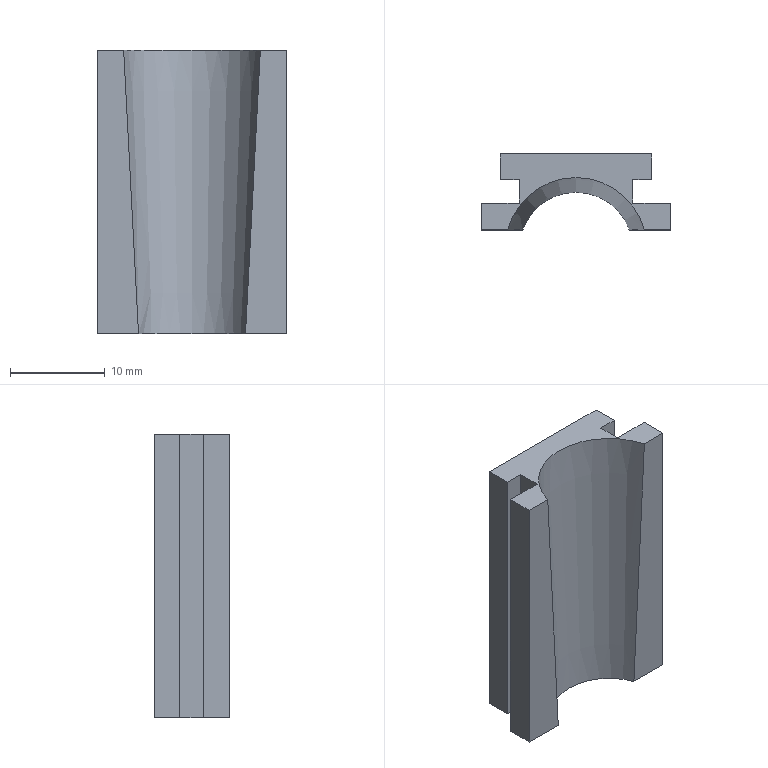Part | 1 solid | 16 faces | box 20 x 8 x 30 mm | volume 2518 mm3 | plane 15 | cone 1
STEP:
#1=CARTESIAN_POINT('',(-6.,1.3,30.));
#2=VERTEX_POINT('',#1);
#3=CARTESIAN_POINT('',(-6.,-1.2,30.));
#4=VERTEX_POINT('',#3);
#5=CARTESIAN_POINT('',(-6.,-1.2,30.));
#6=DIRECTION('',(0.,-1.,0.));
#7=VECTOR('',#6,1000.);
#8=LINE('',#5,#7);
#9=EDGE_CURVE('',#2,#4,#8,.T.);
#10=ORIENTED_EDGE('',*,*,#9,.T.);
#11=CARTESIAN_POINT('',(-10.,-1.2,30.));
#12=VERTEX_POINT('',#11);
#13=CARTESIAN_POINT('',(-10.,-1.2,30.));
#14=DIRECTION('',(-1.,0.,0.));
#15=VECTOR('',#14,1000.);
#16=LINE('',#13,#15);
#17=EDGE_CURVE('',#4,#12,#16,.T.);
#18=ORIENTED_EDGE('',*,*,#17,.T.);
#19=CARTESIAN_POINT('',(-10.,-4.,30.));
#20=VERTEX_POINT('',#19);
#21=CARTESIAN_POINT('',(-10.,-4.,30.));
#22=DIRECTION('',(0.,-1.,0.));
#23=VECTOR('',#22,1000.);
#24=LINE('',#21,#23);
#25=EDGE_CURVE('',#12,#20,#24,.T.);
#26=ORIENTED_EDGE('',*,*,#25,.T.);
#27=CARTESIAN_POINT('',(-7.228,-4.,30.));
#28=VERTEX_POINT('',#27);
#29=CARTESIAN_POINT('',(-10.,-4.,30.));
#30=DIRECTION('',(1.,0.,0.));
#31=VECTOR('',#30,1000.);
#32=LINE('',#29,#31);
#33=EDGE_CURVE('',#20,#28,#32,.T.);
#34=ORIENTED_EDGE('',*,*,#33,.T.);
#35=CARTESIAN_POINT('',(7.228,-4.,30.));
#36=VERTEX_POINT('',#35);
#37=CARTESIAN_POINT('',(0.,-6.,30.));
#38=DIRECTION('',(0.,0.,1.));
#39=DIRECTION('',(1.,0.,0.));
#40=AXIS2_PLACEMENT_3D('',#37,#38,#39);
#41=CIRCLE('',#40,7.5);
#42=EDGE_CURVE('',#36,#28,#41,.T.);
#43=ORIENTED_EDGE('',*,*,#42,.F.);
#44=CARTESIAN_POINT('',(10.,-4.,30.));
#45=VERTEX_POINT('',#44);
#46=CARTESIAN_POINT('',(-10.,-4.,30.));
#47=DIRECTION('',(1.,0.,0.));
#48=VECTOR('',#47,1000.);
#49=LINE('',#46,#48);
#50=EDGE_CURVE('',#36,#45,#49,.T.);
#51=ORIENTED_EDGE('',*,*,#50,.T.);
#52=CARTESIAN_POINT('',(10.,-1.2,30.));
#53=VERTEX_POINT('',#52);
#54=CARTESIAN_POINT('',(10.,-4.,30.));
#55=DIRECTION('',(0.,1.,0.));
#56=VECTOR('',#55,1000.);
#57=LINE('',#54,#56);
#58=EDGE_CURVE('',#45,#53,#57,.T.);
#59=ORIENTED_EDGE('',*,*,#58,.T.);
#60=CARTESIAN_POINT('',(6.,-1.2,30.));
#61=VERTEX_POINT('',#60);
#62=CARTESIAN_POINT('',(10.,-1.2,30.));
#63=DIRECTION('',(-1.,0.,0.));
#64=VECTOR('',#63,1000.);
#65=LINE('',#62,#64);
#66=EDGE_CURVE('',#53,#61,#65,.T.);
#67=ORIENTED_EDGE('',*,*,#66,.T.);
#68=CARTESIAN_POINT('',(6.,1.3,30.));
#69=VERTEX_POINT('',#68);
#70=CARTESIAN_POINT('',(6.,-1.2,30.));
#71=DIRECTION('',(0.,-1.,0.));
#72=VECTOR('',#71,1000.);
#73=LINE('',#70,#72);
#74=EDGE_CURVE('',#69,#61,#73,.T.);
#75=ORIENTED_EDGE('',*,*,#74,.F.);
#76=CARTESIAN_POINT('',(8.,1.3,30.));
#77=VERTEX_POINT('',#76);
#78=CARTESIAN_POINT('',(6.,1.3,30.));
#79=DIRECTION('',(1.,0.,0.));
#80=VECTOR('',#79,1000.);
#81=LINE('',#78,#80);
#82=EDGE_CURVE('',#69,#77,#81,.T.);
#83=ORIENTED_EDGE('',*,*,#82,.T.);
#84=CARTESIAN_POINT('',(8.,4.,30.));
#85=VERTEX_POINT('',#84);
#86=CARTESIAN_POINT('',(8.,-34.067,30.));
#87=DIRECTION('',(0.,1.,0.));
#88=VECTOR('',#87,1000.);
#89=LINE('',#86,#88);
#90=EDGE_CURVE('',#77,#85,#89,.T.);
#91=ORIENTED_EDGE('',*,*,#90,.T.);
#92=CARTESIAN_POINT('',(-8.,4.,30.));
#93=VERTEX_POINT('',#92);
#94=CARTESIAN_POINT('',(-10.,4.,30.));
#95=DIRECTION('',(-1.,0.,0.));
#96=VECTOR('',#95,1000.);
#97=LINE('',#94,#96);
#98=EDGE_CURVE('',#85,#93,#97,.T.);
#99=ORIENTED_EDGE('',*,*,#98,.T.);
#100=CARTESIAN_POINT('',(-8.,1.3,30.));
#101=VERTEX_POINT('',#100);
#102=CARTESIAN_POINT('',(-8.,-34.067,30.));
#103=DIRECTION('',(0.,1.,0.));
#104=VECTOR('',#103,1000.);
#105=LINE('',#102,#104);
#106=EDGE_CURVE('',#101,#93,#105,.T.);
#107=ORIENTED_EDGE('',*,*,#106,.F.);
#108=CARTESIAN_POINT('',(-6.,1.3,30.));
#109=DIRECTION('',(-1.,0.,0.));
#110=VECTOR('',#109,1000.);
#111=LINE('',#108,#110);
#112=EDGE_CURVE('',#2,#101,#111,.T.);
#113=ORIENTED_EDGE('',*,*,#112,.F.);
#114=EDGE_LOOP('',(#10,#18,#26,#34,#43,#51,#59,#67,#75,#83,#91,#99,#107,#113));
#115=FACE_OUTER_BOUND('',#114,.T.);
#116=CARTESIAN_POINT('',(0.,0.,30.));
#117=DIRECTION('',(0.,0.,-1.));
#118=DIRECTION('',(-1.,0.,0.));
#119=AXIS2_PLACEMENT_3D('',#116,#117,#118);
#120=PLANE('',#119);
#121=ADVANCED_FACE('',(#115),#120,.F.);
#122=CARTESIAN_POINT('',(-10.,-1.2,0.));
#123=VERTEX_POINT('',#122);
#124=CARTESIAN_POINT('',(-6.,-1.2,0.));
#125=VERTEX_POINT('',#124);
#126=CARTESIAN_POINT('',(-10.,-1.2,0.));
#127=DIRECTION('',(1.,0.,0.));
#128=VECTOR('',#127,1000.);
#129=LINE('',#126,#128);
#130=EDGE_CURVE('',#123,#125,#129,.T.);
#131=ORIENTED_EDGE('',*,*,#130,.T.);
#132=CARTESIAN_POINT('',(-6.,1.3,0.));
#133=VERTEX_POINT('',#132);
#134=CARTESIAN_POINT('',(-6.,-1.2,0.));
#135=DIRECTION('',(0.,1.,0.));
#136=VECTOR('',#135,1000.);
#137=LINE('',#134,#136);
#138=EDGE_CURVE('',#125,#133,#137,.T.);
#139=ORIENTED_EDGE('',*,*,#138,.T.);
#140=CARTESIAN_POINT('',(-8.,1.3,0.));
#141=VERTEX_POINT('',#140);
#142=CARTESIAN_POINT('',(-6.,1.3,0.));
#143=DIRECTION('',(-1.,0.,0.));
#144=VECTOR('',#143,1000.);
#145=LINE('',#142,#144);
#146=EDGE_CURVE('',#133,#141,#145,.T.);
#147=ORIENTED_EDGE('',*,*,#146,.T.);
#148=CARTESIAN_POINT('',(-8.,4.,0.));
#149=VERTEX_POINT('',#148);
#150=CARTESIAN_POINT('',(-8.,-34.067,0.));
#151=DIRECTION('',(0.,1.,0.));
#152=VECTOR('',#151,1000.);
#153=LINE('',#150,#152);
#154=EDGE_CURVE('',#141,#149,#153,.T.);
#155=ORIENTED_EDGE('',*,*,#154,.T.);
#156=CARTESIAN_POINT('',(8.,4.,0.));
#157=VERTEX_POINT('',#156);
#158=CARTESIAN_POINT('',(-10.,4.,0.));
#159=DIRECTION('',(-1.,0.,0.));
#160=VECTOR('',#159,1000.);
#161=LINE('',#158,#160);
#162=EDGE_CURVE('',#157,#149,#161,.T.);
#163=ORIENTED_EDGE('',*,*,#162,.F.);
#164=CARTESIAN_POINT('',(8.,1.3,0.));
#165=VERTEX_POINT('',#164);
#166=CARTESIAN_POINT('',(8.,-34.067,0.));
#167=DIRECTION('',(0.,1.,0.));
#168=VECTOR('',#167,1000.);
#169=LINE('',#166,#168);
#170=EDGE_CURVE('',#165,#157,#169,.T.);
#171=ORIENTED_EDGE('',*,*,#170,.F.);
#172=CARTESIAN_POINT('',(6.,1.3,0.));
#173=VERTEX_POINT('',#172);
#174=CARTESIAN_POINT('',(6.,1.3,0.));
#175=DIRECTION('',(1.,0.,0.));
#176=VECTOR('',#175,1000.);
#177=LINE('',#174,#176);
#178=EDGE_CURVE('',#173,#165,#177,.T.);
#179=ORIENTED_EDGE('',*,*,#178,.F.);
#180=CARTESIAN_POINT('',(6.,-1.2,0.));
#181=VERTEX_POINT('',#180);
#182=CARTESIAN_POINT('',(6.,-1.2,0.));
#183=DIRECTION('',(0.,1.,0.));
#184=VECTOR('',#183,1000.);
#185=LINE('',#182,#184);
#186=EDGE_CURVE('',#181,#173,#185,.T.);
#187=ORIENTED_EDGE('',*,*,#186,.F.);
#188=CARTESIAN_POINT('',(10.,-1.2,0.));
#189=VERTEX_POINT('',#188);
#190=CARTESIAN_POINT('',(10.,-1.2,0.));
#191=DIRECTION('',(1.,0.,0.));
#192=VECTOR('',#191,1000.);
#193=LINE('',#190,#192);
#194=EDGE_CURVE('',#181,#189,#193,.T.);
#195=ORIENTED_EDGE('',*,*,#194,.T.);
#196=CARTESIAN_POINT('',(10.,-4.,0.));
#197=VERTEX_POINT('',#196);
#198=CARTESIAN_POINT('',(10.,-4.,0.));
#199=DIRECTION('',(0.,1.,0.));
#200=VECTOR('',#199,1000.);
#201=LINE('',#198,#200);
#202=EDGE_CURVE('',#197,#189,#201,.T.);
#203=ORIENTED_EDGE('',*,*,#202,.F.);
#204=CARTESIAN_POINT('',(5.657,-4.,0.));
#205=VERTEX_POINT('',#204);
#206=CARTESIAN_POINT('',(-10.,-4.,0.));
#207=DIRECTION('',(1.,0.,0.));
#208=VECTOR('',#207,1000.);
#209=LINE('',#206,#208);
#210=EDGE_CURVE('',#205,#197,#209,.T.);
#211=ORIENTED_EDGE('',*,*,#210,.F.);
#212=CARTESIAN_POINT('',(-5.657,-4.,0.));
#213=VERTEX_POINT('',#212);
#214=CARTESIAN_POINT('',(0.,-6.,0.));
#215=DIRECTION('',(0.,0.,1.));
#216=DIRECTION('',(1.,0.,0.));
#217=AXIS2_PLACEMENT_3D('',#214,#215,#216);
#218=CIRCLE('',#217,6.);
#219=EDGE_CURVE('',#205,#213,#218,.T.);
#220=ORIENTED_EDGE('',*,*,#219,.T.);
#221=CARTESIAN_POINT('',(-10.,-4.,0.));
#222=VERTEX_POINT('',#221);
#223=CARTESIAN_POINT('',(-10.,-4.,0.));
#224=DIRECTION('',(1.,0.,0.));
#225=VECTOR('',#224,1000.);
#226=LINE('',#223,#225);
#227=EDGE_CURVE('',#222,#213,#226,.T.);
#228=ORIENTED_EDGE('',*,*,#227,.F.);
#229=CARTESIAN_POINT('',(-10.,-4.,0.));
#230=DIRECTION('',(0.,-1.,0.));
#231=VECTOR('',#230,1000.);
#232=LINE('',#229,#231);
#233=EDGE_CURVE('',#123,#222,#232,.T.);
#234=ORIENTED_EDGE('',*,*,#233,.F.);
#235=EDGE_LOOP('',(#131,#139,#147,#155,#163,#171,#179,#187,#195,#203,#211,#220,#228,#234));
#236=FACE_OUTER_BOUND('',#235,.T.);
#237=CARTESIAN_POINT('',(0.,0.,0.));
#238=DIRECTION('',(0.,0.,-1.));
#239=DIRECTION('',(-1.,0.,0.));
#240=AXIS2_PLACEMENT_3D('',#237,#238,#239);
#241=PLANE('',#240);
#242=ADVANCED_FACE('',(#236),#241,.T.);
#243=CARTESIAN_POINT('',(-8.,1.3,30.));
#244=DIRECTION('',(0.,0.,1.));
#245=VECTOR('',#244,1000.);
#246=LINE('',#243,#245);
#247=EDGE_CURVE('',#141,#101,#246,.T.);
#248=ORIENTED_EDGE('',*,*,#247,.T.);
#249=ORIENTED_EDGE('',*,*,#106,.T.);
#250=CARTESIAN_POINT('',(-8.,4.,0.));
#251=DIRECTION('',(0.,0.,-1.));
#252=VECTOR('',#251,1000.);
#253=LINE('',#250,#252);
#254=EDGE_CURVE('',#93,#149,#253,.T.);
#255=ORIENTED_EDGE('',*,*,#254,.T.);
#256=ORIENTED_EDGE('',*,*,#154,.F.);
#257=EDGE_LOOP('',(#248,#249,#255,#256));
#258=FACE_OUTER_BOUND('',#257,.T.);
#259=CARTESIAN_POINT('',(-8.,-34.067,0.));
#260=DIRECTION('',(1.,0.,0.));
#261=DIRECTION('',(0.,0.,-1.));
#262=AXIS2_PLACEMENT_3D('',#259,#260,#261);
#263=PLANE('',#262);
#264=ADVANCED_FACE('',(#258),#263,.F.);
#265=CARTESIAN_POINT('',(-7.228,-4.,30.));
#266=CARTESIAN_POINT('',(-6.71,-4.,20.));
#267=CARTESIAN_POINT('',(-6.187,-4.,10.));
#268=CARTESIAN_POINT('',(-5.657,-4.,0.));
#269=B_SPLINE_CURVE_WITH_KNOTS('',3,(#265,#266,#267,#268),.UNSPECIFIED.,.F.,.F.,(4,4),(0.02987,0.05991),.UNSPECIFIED.);
#270=EDGE_CURVE('',#28,#213,#269,.T.);
#271=ORIENTED_EDGE('',*,*,#270,.F.);
#272=ORIENTED_EDGE('',*,*,#33,.F.);
#273=CARTESIAN_POINT('',(-10.,-4.,30.));
#274=DIRECTION('',(0.,0.,-1.));
#275=VECTOR('',#274,1000.);
#276=LINE('',#273,#275);
#277=EDGE_CURVE('',#20,#222,#276,.T.);
#278=ORIENTED_EDGE('',*,*,#277,.T.);
#279=ORIENTED_EDGE('',*,*,#227,.T.);
#280=EDGE_LOOP('',(#271,#272,#278,#279));
#281=FACE_OUTER_BOUND('',#280,.T.);
#282=CARTESIAN_POINT('',(-10.,-4.,30.));
#283=DIRECTION('',(0.,1.,0.));
#284=DIRECTION('',(0.,0.,1.));
#285=AXIS2_PLACEMENT_3D('',#282,#283,#284);
#286=PLANE('',#285);
#287=ADVANCED_FACE('',(#281),#286,.F.);
#288=CARTESIAN_POINT('',(5.657,-4.,0.));
#289=CARTESIAN_POINT('',(6.187,-4.,10.));
#290=CARTESIAN_POINT('',(6.71,-4.,20.));
#291=CARTESIAN_POINT('',(7.228,-4.,30.));
#292=B_SPLINE_CURVE_WITH_KNOTS('',3,(#288,#289,#290,#291),.UNSPECIFIED.,.F.,.F.,(4,4),(0.05617,0.08621),.UNSPECIFIED.);
#293=EDGE_CURVE('',#205,#36,#292,.T.);
#294=ORIENTED_EDGE('',*,*,#293,.F.);
#295=ORIENTED_EDGE('',*,*,#210,.T.);
#296=CARTESIAN_POINT('',(10.,-4.,30.));
#297=DIRECTION('',(0.,0.,-1.));
#298=VECTOR('',#297,1000.);
#299=LINE('',#296,#298);
#300=EDGE_CURVE('',#45,#197,#299,.T.);
#301=ORIENTED_EDGE('',*,*,#300,.F.);
#302=ORIENTED_EDGE('',*,*,#50,.F.);
#303=EDGE_LOOP('',(#294,#295,#301,#302));
#304=FACE_OUTER_BOUND('',#303,.T.);
#305=CARTESIAN_POINT('',(-10.,-4.,30.));
#306=DIRECTION('',(0.,1.,0.));
#307=DIRECTION('',(0.,0.,1.));
#308=AXIS2_PLACEMENT_3D('',#305,#306,#307);
#309=PLANE('',#308);
#310=ADVANCED_FACE('',(#304),#309,.F.);
#311=CARTESIAN_POINT('',(10.,-1.2,0.));
#312=DIRECTION('',(0.,0.,1.));
#313=VECTOR('',#312,1000.);
#314=LINE('',#311,#313);
#315=EDGE_CURVE('',#189,#53,#314,.T.);
#316=ORIENTED_EDGE('',*,*,#315,.T.);
#317=ORIENTED_EDGE('',*,*,#58,.F.);
#318=ORIENTED_EDGE('',*,*,#300,.T.);
#319=ORIENTED_EDGE('',*,*,#202,.T.);
#320=EDGE_LOOP('',(#316,#317,#318,#319));
#321=FACE_OUTER_BOUND('',#320,.T.);
#322=CARTESIAN_POINT('',(10.,-4.,30.));
#323=DIRECTION('',(-1.,0.,0.));
#324=DIRECTION('',(0.,0.,1.));
#325=AXIS2_PLACEMENT_3D('',#322,#323,#324);
#326=PLANE('',#325);
#327=ADVANCED_FACE('',(#321),#326,.F.);
#328=CARTESIAN_POINT('',(-10.,-1.2,0.));
#329=DIRECTION('',(0.,0.,-1.));
#330=VECTOR('',#329,1000.);
#331=LINE('',#328,#330);
#332=EDGE_CURVE('',#12,#123,#331,.T.);
#333=ORIENTED_EDGE('',*,*,#332,.T.);
#334=ORIENTED_EDGE('',*,*,#233,.T.);
#335=ORIENTED_EDGE('',*,*,#277,.F.);
#336=ORIENTED_EDGE('',*,*,#25,.F.);
#337=EDGE_LOOP('',(#333,#334,#335,#336));
#338=FACE_OUTER_BOUND('',#337,.T.);
#339=CARTESIAN_POINT('',(-10.,-4.,30.));
#340=DIRECTION('',(1.,0.,0.));
#341=DIRECTION('',(0.,0.,-1.));
#342=AXIS2_PLACEMENT_3D('',#339,#340,#341);
#343=PLANE('',#342);
#344=ADVANCED_FACE('',(#338),#343,.F.);
#345=ORIENTED_EDGE('',*,*,#98,.F.);
#346=CARTESIAN_POINT('',(8.,4.,0.));
#347=DIRECTION('',(0.,0.,1.));
#348=VECTOR('',#347,1000.);
#349=LINE('',#346,#348);
#350=EDGE_CURVE('',#157,#85,#349,.T.);
#351=ORIENTED_EDGE('',*,*,#350,.F.);
#352=ORIENTED_EDGE('',*,*,#162,.T.);
#353=ORIENTED_EDGE('',*,*,#254,.F.);
#354=EDGE_LOOP('',(#345,#351,#352,#353));
#355=FACE_OUTER_BOUND('',#354,.T.);
#356=CARTESIAN_POINT('',(-10.,4.,30.));
#357=DIRECTION('',(0.,-1.,0.));
#358=DIRECTION('',(0.,0.,-1.));
#359=AXIS2_PLACEMENT_3D('',#356,#357,#358);
#360=PLANE('',#359);
#361=ADVANCED_FACE('',(#355),#360,.F.);
#362=ORIENTED_EDGE('',*,*,#332,.F.);
#363=ORIENTED_EDGE('',*,*,#17,.F.);
#364=CARTESIAN_POINT('',(-6.,-1.2,30.));
#365=DIRECTION('',(0.,0.,-1.));
#366=VECTOR('',#365,1000.);
#367=LINE('',#364,#366);
#368=EDGE_CURVE('',#4,#125,#367,.T.);
#369=ORIENTED_EDGE('',*,*,#368,.T.);
#370=ORIENTED_EDGE('',*,*,#130,.F.);
#371=EDGE_LOOP('',(#362,#363,#369,#370));
#372=FACE_OUTER_BOUND('',#371,.T.);
#373=CARTESIAN_POINT('',(-10.,-1.2,30.));
#374=DIRECTION('',(0.,1.,0.));
#375=DIRECTION('',(0.,0.,1.));
#376=AXIS2_PLACEMENT_3D('',#373,#374,#375);
#377=PLANE('',#376);
#378=ADVANCED_FACE('',(#372),#377,.T.);
#379=ORIENTED_EDGE('',*,*,#90,.F.);
#380=CARTESIAN_POINT('',(8.,1.3,30.));
#381=DIRECTION('',(0.,0.,1.));
#382=VECTOR('',#381,1000.);
#383=LINE('',#380,#382);
#384=EDGE_CURVE('',#165,#77,#383,.T.);
#385=ORIENTED_EDGE('',*,*,#384,.F.);
#386=ORIENTED_EDGE('',*,*,#170,.T.);
#387=ORIENTED_EDGE('',*,*,#350,.T.);
#388=EDGE_LOOP('',(#379,#385,#386,#387));
#389=FACE_OUTER_BOUND('',#388,.T.);
#390=CARTESIAN_POINT('',(8.,-34.067,0.));
#391=DIRECTION('',(-1.,0.,0.));
#392=DIRECTION('',(0.,0.,1.));
#393=AXIS2_PLACEMENT_3D('',#390,#391,#392);
#394=PLANE('',#393);
#395=ADVANCED_FACE('',(#389),#394,.F.);
#396=ORIENTED_EDGE('',*,*,#315,.F.);
#397=ORIENTED_EDGE('',*,*,#194,.F.);
#398=CARTESIAN_POINT('',(6.,-1.2,30.));
#399=DIRECTION('',(0.,0.,-1.));
#400=VECTOR('',#399,1000.);
#401=LINE('',#398,#400);
#402=EDGE_CURVE('',#61,#181,#401,.T.);
#403=ORIENTED_EDGE('',*,*,#402,.F.);
#404=ORIENTED_EDGE('',*,*,#66,.F.);
#405=EDGE_LOOP('',(#396,#397,#403,#404));
#406=FACE_OUTER_BOUND('',#405,.T.);
#407=CARTESIAN_POINT('',(-10.,-1.2,30.));
#408=DIRECTION('',(0.,1.,0.));
#409=DIRECTION('',(0.,0.,1.));
#410=AXIS2_PLACEMENT_3D('',#407,#408,#409);
#411=PLANE('',#410);
#412=ADVANCED_FACE('',(#406),#411,.T.);
#413=ORIENTED_EDGE('',*,*,#384,.T.);
#414=ORIENTED_EDGE('',*,*,#82,.F.);
#415=CARTESIAN_POINT('',(6.,1.3,30.));
#416=DIRECTION('',(0.,0.,1.));
#417=VECTOR('',#416,1000.);
#418=LINE('',#415,#417);
#419=EDGE_CURVE('',#173,#69,#418,.T.);
#420=ORIENTED_EDGE('',*,*,#419,.F.);
#421=ORIENTED_EDGE('',*,*,#178,.T.);
#422=EDGE_LOOP('',(#413,#414,#420,#421));
#423=FACE_OUTER_BOUND('',#422,.T.);
#424=CARTESIAN_POINT('',(6.,1.3,30.));
#425=DIRECTION('',(0.,1.,0.));
#426=DIRECTION('',(0.,0.,1.));
#427=AXIS2_PLACEMENT_3D('',#424,#425,#426);
#428=PLANE('',#427);
#429=ADVANCED_FACE('',(#423),#428,.F.);
#430=ORIENTED_EDGE('',*,*,#74,.T.);
#431=ORIENTED_EDGE('',*,*,#402,.T.);
#432=ORIENTED_EDGE('',*,*,#186,.T.);
#433=ORIENTED_EDGE('',*,*,#419,.T.);
#434=EDGE_LOOP('',(#430,#431,#432,#433));
#435=FACE_OUTER_BOUND('',#434,.T.);
#436=CARTESIAN_POINT('',(6.,0.,0.));
#437=DIRECTION('',(-1.,0.,0.));
#438=DIRECTION('',(0.,0.,1.));
#439=AXIS2_PLACEMENT_3D('',#436,#437,#438);
#440=PLANE('',#439);
#441=ADVANCED_FACE('',(#435),#440,.F.);
#442=ORIENTED_EDGE('',*,*,#270,.T.);
#443=ORIENTED_EDGE('',*,*,#219,.F.);
#444=ORIENTED_EDGE('',*,*,#293,.T.);
#445=ORIENTED_EDGE('',*,*,#42,.T.);
#446=EDGE_LOOP('',(#442,#443,#444,#445));
#447=FACE_OUTER_BOUND('',#446,.T.);
#448=CARTESIAN_POINT('',(0.,-6.,0.));
#449=DIRECTION('',(0.,0.,1.));
#450=DIRECTION('',(1.,0.,0.));
#451=AXIS2_PLACEMENT_3D('',#448,#449,#450);
#452=CONICAL_SURFACE('',#451,6.,0.04996);
#453=ADVANCED_FACE('',(#447),#452,.F.);
#454=ORIENTED_EDGE('',*,*,#247,.F.);
#455=ORIENTED_EDGE('',*,*,#146,.F.);
#456=CARTESIAN_POINT('',(-6.,1.3,30.));
#457=DIRECTION('',(0.,0.,1.));
#458=VECTOR('',#457,1000.);
#459=LINE('',#456,#458);
#460=EDGE_CURVE('',#133,#2,#459,.T.);
#461=ORIENTED_EDGE('',*,*,#460,.T.);
#462=ORIENTED_EDGE('',*,*,#112,.T.);
#463=EDGE_LOOP('',(#454,#455,#461,#462));
#464=FACE_OUTER_BOUND('',#463,.T.);
#465=CARTESIAN_POINT('',(-6.,1.3,30.));
#466=DIRECTION('',(0.,-1.,0.));
#467=DIRECTION('',(0.,0.,-1.));
#468=AXIS2_PLACEMENT_3D('',#465,#466,#467);
#469=PLANE('',#468);
#470=ADVANCED_FACE('',(#464),#469,.T.);
#471=ORIENTED_EDGE('',*,*,#9,.F.);
#472=ORIENTED_EDGE('',*,*,#460,.F.);
#473=ORIENTED_EDGE('',*,*,#138,.F.);
#474=ORIENTED_EDGE('',*,*,#368,.F.);
#475=EDGE_LOOP('',(#471,#472,#473,#474));
#476=FACE_OUTER_BOUND('',#475,.T.);
#477=CARTESIAN_POINT('',(-6.,0.,0.));
#478=DIRECTION('',(1.,0.,0.));
#479=DIRECTION('',(0.,0.,1.));
#480=AXIS2_PLACEMENT_3D('',#477,#478,#479);
#481=PLANE('',#480);
#482=ADVANCED_FACE('',(#476),#481,.F.);
#483=CLOSED_SHELL('',(#121,#242,#264,#287,#310,#327,#344,#361,#378,#395,#412,#429,#441,#453,#470,#482));
#484=MANIFOLD_SOLID_BREP('',#483);
#485=CARTESIAN_POINT('',(0.,0.,0.));
#486=DIRECTION('',(0.,0.,1.));
#487=DIRECTION('',(1.,0.,0.));
#488=AXIS2_PLACEMENT_3D('',#485,#486,#487);
#489=(LENGTH_UNIT()NAMED_UNIT(*)SI_UNIT(.MILLI.,.METRE.));
#490=UNCERTAINTY_MEASURE_WITH_UNIT(LENGTH_MEASURE(0.00001),#489,'','');
#491=(NAMED_UNIT(*)PLANE_ANGLE_UNIT()SI_UNIT($,.RADIAN.));
#492=(NAMED_UNIT(*)SI_UNIT($,.STERADIAN.)SOLID_ANGLE_UNIT());
#493=(GEOMETRIC_REPRESENTATION_CONTEXT(3)GLOBAL_UNCERTAINTY_ASSIGNED_CONTEXT((#490))GLOBAL_UNIT_ASSIGNED_CONTEXT((#489,#491,#492))REPRESENTATION_CONTEXT('',''));
#494=ADVANCED_BREP_SHAPE_REPRESENTATION('',(#484,#488),#493);